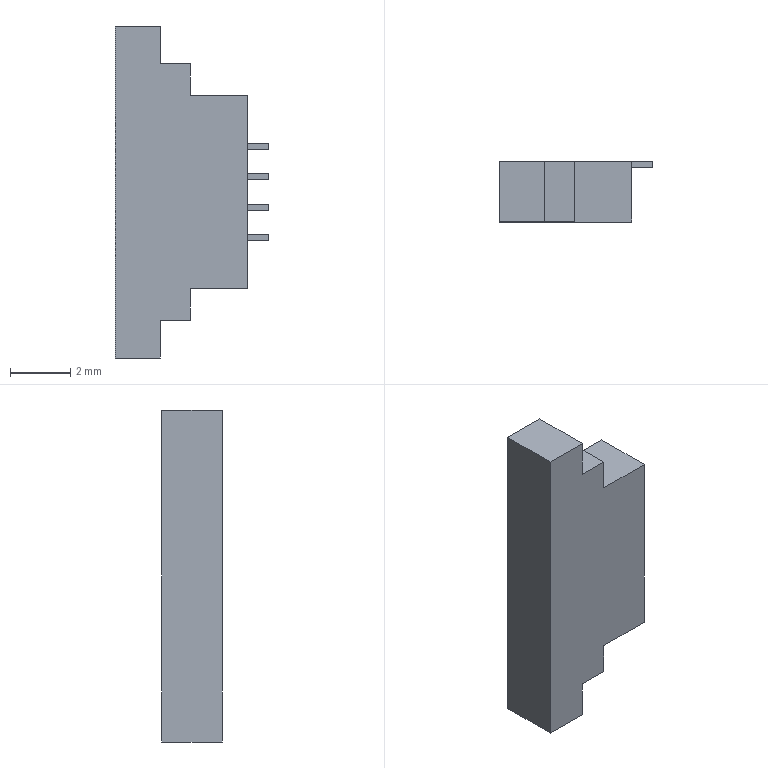Part | SolidWorks | features BaseBody 1 | 1 solid | 30 faces | box 5.1 x 2 x 11 mm | volume 74.432 mm3 | plane 30
STEP:
#1=CARTESIAN_POINT('',(-66.9,-34.61,-10.6));
#2=VERTEX_POINT('',#1);
#3=CARTESIAN_POINT('',(-67.6,-34.61,-10.6));
#4=VERTEX_POINT('',#3);
#5=CARTESIAN_POINT('',(-69.45,-34.61,-10.6));
#6=DIRECTION('',(-1.,0.,0.));
#7=VECTOR('',#6,1000.);
#8=LINE('',#5,#7);
#9=EDGE_CURVE('',#2,#4,#8,.T.);
#10=ORIENTED_EDGE('',*,*,#9,.T.);
#11=CARTESIAN_POINT('',(-67.6,-34.61,-11.4));
#12=VERTEX_POINT('',#11);
#13=CARTESIAN_POINT('',(-67.6,-34.61,-12.));
#14=DIRECTION('',(0.,0.,1.));
#15=VECTOR('',#14,1000.);
#16=LINE('',#13,#15);
#17=EDGE_CURVE('',#12,#4,#16,.T.);
#18=ORIENTED_EDGE('',*,*,#17,.F.);
#19=CARTESIAN_POINT('',(-66.9,-34.61,-11.4));
#20=VERTEX_POINT('',#19);
#21=CARTESIAN_POINT('',(-69.45,-34.61,-11.4));
#22=DIRECTION('',(1.,0.,0.));
#23=VECTOR('',#22,1000.);
#24=LINE('',#21,#23);
#25=EDGE_CURVE('',#12,#20,#24,.T.);
#26=ORIENTED_EDGE('',*,*,#25,.T.);
#27=CARTESIAN_POINT('',(-66.9,-34.61,-11.6));
#28=VERTEX_POINT('',#27);
#29=CARTESIAN_POINT('',(-66.9,-34.61,-12.));
#30=DIRECTION('',(0.,0.,-1.));
#31=VECTOR('',#30,1000.);
#32=LINE('',#29,#31);
#33=EDGE_CURVE('',#20,#28,#32,.T.);
#34=ORIENTED_EDGE('',*,*,#33,.T.);
#35=CARTESIAN_POINT('',(-67.6,-34.61,-11.6));
#36=VERTEX_POINT('',#35);
#37=CARTESIAN_POINT('',(-69.45,-34.61,-11.6));
#38=DIRECTION('',(-1.,0.,0.));
#39=VECTOR('',#38,1000.);
#40=LINE('',#37,#39);
#41=EDGE_CURVE('',#28,#36,#40,.T.);
#42=ORIENTED_EDGE('',*,*,#41,.T.);
#43=CARTESIAN_POINT('',(-67.6,-34.61,-12.4));
#44=VERTEX_POINT('',#43);
#45=CARTESIAN_POINT('',(-67.6,-34.61,-12.));
#46=DIRECTION('',(0.,0.,1.));
#47=VECTOR('',#46,1000.);
#48=LINE('',#45,#47);
#49=EDGE_CURVE('',#44,#36,#48,.T.);
#50=ORIENTED_EDGE('',*,*,#49,.F.);
#51=CARTESIAN_POINT('',(-66.9,-34.61,-12.4));
#52=VERTEX_POINT('',#51);
#53=CARTESIAN_POINT('',(-69.45,-34.61,-12.4));
#54=DIRECTION('',(1.,0.,0.));
#55=VECTOR('',#54,1000.);
#56=LINE('',#53,#55);
#57=EDGE_CURVE('',#44,#52,#56,.T.);
#58=ORIENTED_EDGE('',*,*,#57,.T.);
#59=CARTESIAN_POINT('',(-66.9,-34.61,-12.6));
#60=VERTEX_POINT('',#59);
#61=CARTESIAN_POINT('',(-66.9,-34.61,-12.));
#62=DIRECTION('',(0.,0.,-1.));
#63=VECTOR('',#62,1000.);
#64=LINE('',#61,#63);
#65=EDGE_CURVE('',#52,#60,#64,.T.);
#66=ORIENTED_EDGE('',*,*,#65,.T.);
#67=CARTESIAN_POINT('',(-67.6,-34.61,-12.6));
#68=VERTEX_POINT('',#67);
#69=CARTESIAN_POINT('',(-69.45,-34.61,-12.6));
#70=DIRECTION('',(-1.,0.,0.));
#71=VECTOR('',#70,1000.);
#72=LINE('',#69,#71);
#73=EDGE_CURVE('',#60,#68,#72,.T.);
#74=ORIENTED_EDGE('',*,*,#73,.T.);
#75=CARTESIAN_POINT('',(-67.6,-34.61,-13.4));
#76=VERTEX_POINT('',#75);
#77=CARTESIAN_POINT('',(-67.6,-34.61,-12.));
#78=DIRECTION('',(0.,0.,1.));
#79=VECTOR('',#78,1000.);
#80=LINE('',#77,#79);
#81=EDGE_CURVE('',#76,#68,#80,.T.);
#82=ORIENTED_EDGE('',*,*,#81,.F.);
#83=CARTESIAN_POINT('',(-66.9,-34.61,-13.4));
#84=VERTEX_POINT('',#83);
#85=CARTESIAN_POINT('',(-69.45,-34.61,-13.4));
#86=DIRECTION('',(1.,0.,0.));
#87=VECTOR('',#86,1000.);
#88=LINE('',#85,#87);
#89=EDGE_CURVE('',#76,#84,#88,.T.);
#90=ORIENTED_EDGE('',*,*,#89,.T.);
#91=CARTESIAN_POINT('',(-66.9,-34.61,-13.6));
#92=VERTEX_POINT('',#91);
#93=CARTESIAN_POINT('',(-66.9,-34.61,-12.));
#94=DIRECTION('',(0.,0.,-1.));
#95=VECTOR('',#94,1000.);
#96=LINE('',#93,#95);
#97=EDGE_CURVE('',#84,#92,#96,.T.);
#98=ORIENTED_EDGE('',*,*,#97,.T.);
#99=CARTESIAN_POINT('',(-67.6,-34.61,-13.6));
#100=VERTEX_POINT('',#99);
#101=CARTESIAN_POINT('',(-69.45,-34.61,-13.6));
#102=DIRECTION('',(-1.,0.,0.));
#103=VECTOR('',#102,1000.);
#104=LINE('',#101,#103);
#105=EDGE_CURVE('',#92,#100,#104,.T.);
#106=ORIENTED_EDGE('',*,*,#105,.T.);
#107=CARTESIAN_POINT('',(-67.6,-34.61,-15.2));
#108=VERTEX_POINT('',#107);
#109=CARTESIAN_POINT('',(-67.6,-34.61,-12.));
#110=DIRECTION('',(0.,0.,1.));
#111=VECTOR('',#110,1000.);
#112=LINE('',#109,#111);
#113=EDGE_CURVE('',#108,#100,#112,.T.);
#114=ORIENTED_EDGE('',*,*,#113,.F.);
#115=CARTESIAN_POINT('',(-69.5,-34.61,-15.2));
#116=VERTEX_POINT('',#115);
#117=CARTESIAN_POINT('',(-69.45,-34.61,-15.2));
#118=DIRECTION('',(-1.,0.,0.));
#119=VECTOR('',#118,1000.);
#120=LINE('',#117,#119);
#121=EDGE_CURVE('',#108,#116,#120,.T.);
#122=ORIENTED_EDGE('',*,*,#121,.T.);
#123=CARTESIAN_POINT('',(-69.5,-34.61,-16.25));
#124=VERTEX_POINT('',#123);
#125=CARTESIAN_POINT('',(-69.5,-34.61,-15.725));
#126=DIRECTION('',(0.,0.,1.));
#127=VECTOR('',#126,1000.);
#128=LINE('',#125,#127);
#129=EDGE_CURVE('',#124,#116,#128,.T.);
#130=ORIENTED_EDGE('',*,*,#129,.F.);
#131=CARTESIAN_POINT('',(-70.5,-34.61,-16.25));
#132=VERTEX_POINT('',#131);
#133=CARTESIAN_POINT('',(-70.,-34.61,-16.25));
#134=DIRECTION('',(-1.,0.,0.));
#135=VECTOR('',#134,1000.);
#136=LINE('',#133,#135);
#137=EDGE_CURVE('',#124,#132,#136,.T.);
#138=ORIENTED_EDGE('',*,*,#137,.T.);
#139=CARTESIAN_POINT('',(-70.5,-34.61,-17.5));
#140=VERTEX_POINT('',#139);
#141=CARTESIAN_POINT('',(-70.5,-34.61,-16.875));
#142=DIRECTION('',(0.,0.,1.));
#143=VECTOR('',#142,1000.);
#144=LINE('',#141,#143);
#145=EDGE_CURVE('',#140,#132,#144,.T.);
#146=ORIENTED_EDGE('',*,*,#145,.F.);
#147=CARTESIAN_POINT('',(-72.,-34.61,-17.5));
#148=VERTEX_POINT('',#147);
#149=CARTESIAN_POINT('',(-71.25,-34.61,-17.5));
#150=DIRECTION('',(-1.,0.,0.));
#151=VECTOR('',#150,1000.);
#152=LINE('',#149,#151);
#153=EDGE_CURVE('',#140,#148,#152,.T.);
#154=ORIENTED_EDGE('',*,*,#153,.T.);
#155=CARTESIAN_POINT('',(-72.,-34.61,-6.5));
#156=VERTEX_POINT('',#155);
#157=CARTESIAN_POINT('',(-72.,-34.61,-12.));
#158=DIRECTION('',(0.,0.,1.));
#159=VECTOR('',#158,1000.);
#160=LINE('',#157,#159);
#161=EDGE_CURVE('',#148,#156,#160,.T.);
#162=ORIENTED_EDGE('',*,*,#161,.T.);
#163=CARTESIAN_POINT('',(-70.5,-34.61,-6.5));
#164=VERTEX_POINT('',#163);
#165=CARTESIAN_POINT('',(-71.25,-34.61,-6.5));
#166=DIRECTION('',(-1.,0.,0.));
#167=VECTOR('',#166,1000.);
#168=LINE('',#165,#167);
#169=EDGE_CURVE('',#164,#156,#168,.T.);
#170=ORIENTED_EDGE('',*,*,#169,.F.);
#171=CARTESIAN_POINT('',(-70.5,-34.61,-7.75));
#172=VERTEX_POINT('',#171);
#173=CARTESIAN_POINT('',(-70.5,-34.61,-7.125));
#174=DIRECTION('',(0.,0.,1.));
#175=VECTOR('',#174,1000.);
#176=LINE('',#173,#175);
#177=EDGE_CURVE('',#172,#164,#176,.T.);
#178=ORIENTED_EDGE('',*,*,#177,.F.);
#179=CARTESIAN_POINT('',(-69.5,-34.61,-7.75));
#180=VERTEX_POINT('',#179);
#181=CARTESIAN_POINT('',(-70.,-34.61,-7.75));
#182=DIRECTION('',(-1.,0.,0.));
#183=VECTOR('',#182,1000.);
#184=LINE('',#181,#183);
#185=EDGE_CURVE('',#180,#172,#184,.T.);
#186=ORIENTED_EDGE('',*,*,#185,.F.);
#187=CARTESIAN_POINT('',(-69.5,-34.61,-8.8));
#188=VERTEX_POINT('',#187);
#189=CARTESIAN_POINT('',(-69.5,-34.61,-8.275));
#190=DIRECTION('',(0.,0.,1.));
#191=VECTOR('',#190,1000.);
#192=LINE('',#189,#191);
#193=EDGE_CURVE('',#188,#180,#192,.T.);
#194=ORIENTED_EDGE('',*,*,#193,.F.);
#195=CARTESIAN_POINT('',(-67.6,-34.61,-8.8));
#196=VERTEX_POINT('',#195);
#197=CARTESIAN_POINT('',(-69.45,-34.61,-8.8));
#198=DIRECTION('',(1.,0.,0.));
#199=VECTOR('',#198,1000.);
#200=LINE('',#197,#199);
#201=EDGE_CURVE('',#188,#196,#200,.T.);
#202=ORIENTED_EDGE('',*,*,#201,.T.);
#203=CARTESIAN_POINT('',(-67.6,-34.61,-10.4));
#204=VERTEX_POINT('',#203);
#205=CARTESIAN_POINT('',(-67.6,-34.61,-12.));
#206=DIRECTION('',(0.,0.,1.));
#207=VECTOR('',#206,1000.);
#208=LINE('',#205,#207);
#209=EDGE_CURVE('',#204,#196,#208,.T.);
#210=ORIENTED_EDGE('',*,*,#209,.F.);
#211=CARTESIAN_POINT('',(-66.9,-34.61,-10.4));
#212=VERTEX_POINT('',#211);
#213=CARTESIAN_POINT('',(-69.45,-34.61,-10.4));
#214=DIRECTION('',(1.,0.,0.));
#215=VECTOR('',#214,1000.);
#216=LINE('',#213,#215);
#217=EDGE_CURVE('',#204,#212,#216,.T.);
#218=ORIENTED_EDGE('',*,*,#217,.T.);
#219=CARTESIAN_POINT('',(-66.9,-34.61,-12.));
#220=DIRECTION('',(0.,0.,-1.));
#221=VECTOR('',#220,1000.);
#222=LINE('',#219,#221);
#223=EDGE_CURVE('',#212,#2,#222,.T.);
#224=ORIENTED_EDGE('',*,*,#223,.T.);
#225=EDGE_LOOP('',(#10,#18,#26,#34,#42,#50,#58,#66,#74,#82,#90,#98,#106,#114,#122,#130,#138,#146,#154,#162,#170,#178,#186,#194,#202,#210,#218,#224));
#226=FACE_OUTER_BOUND('',#225,.T.);
#227=CARTESIAN_POINT('',(-69.45,-34.61,-12.));
#228=DIRECTION('',(0.,1.,0.));
#229=DIRECTION('',(0.,0.,1.));
#230=AXIS2_PLACEMENT_3D('',#227,#228,#229);
#231=PLANE('',#230);
#232=ADVANCED_FACE('',(#226),#231,.T.);
#233=CARTESIAN_POINT('',(-66.9,-34.81,-10.6));
#234=VERTEX_POINT('',#233);
#235=CARTESIAN_POINT('',(-66.9,-34.71,-10.6));
#236=DIRECTION('',(0.,1.,0.));
#237=VECTOR('',#236,1000.);
#238=LINE('',#235,#237);
#239=EDGE_CURVE('',#234,#2,#238,.T.);
#240=ORIENTED_EDGE('',*,*,#239,.F.);
#241=CARTESIAN_POINT('',(-67.6,-34.81,-10.6));
#242=VERTEX_POINT('',#241);
#243=CARTESIAN_POINT('',(-67.25,-34.81,-10.6));
#244=DIRECTION('',(1.,0.,0.));
#245=VECTOR('',#244,1000.);
#246=LINE('',#243,#245);
#247=EDGE_CURVE('',#242,#234,#246,.T.);
#248=ORIENTED_EDGE('',*,*,#247,.F.);
#249=CARTESIAN_POINT('',(-67.6,-35.61,-10.6));
#250=DIRECTION('',(0.,-1.,0.));
#251=VECTOR('',#250,1000.);
#252=LINE('',#249,#251);
#253=EDGE_CURVE('',#4,#242,#252,.T.);
#254=ORIENTED_EDGE('',*,*,#253,.F.);
#255=ORIENTED_EDGE('',*,*,#9,.F.);
#256=EDGE_LOOP('',(#240,#248,#254,#255));
#257=FACE_OUTER_BOUND('',#256,.T.);
#258=CARTESIAN_POINT('',(-67.25,-34.71,-10.6));
#259=DIRECTION('',(0.,0.,1.));
#260=DIRECTION('',(1.,0.,0.));
#261=AXIS2_PLACEMENT_3D('',#258,#259,#260);
#262=PLANE('',#261);
#263=ADVANCED_FACE('',(#257),#262,.F.);
#264=ORIENTED_EDGE('',*,*,#239,.T.);
#265=ORIENTED_EDGE('',*,*,#223,.F.);
#266=CARTESIAN_POINT('',(-66.9,-34.81,-10.4));
#267=VERTEX_POINT('',#266);
#268=CARTESIAN_POINT('',(-66.9,-34.71,-10.4));
#269=DIRECTION('',(0.,-1.,0.));
#270=VECTOR('',#269,1000.);
#271=LINE('',#268,#270);
#272=EDGE_CURVE('',#212,#267,#271,.T.);
#273=ORIENTED_EDGE('',*,*,#272,.T.);
#274=CARTESIAN_POINT('',(-66.9,-34.81,-10.5));
#275=DIRECTION('',(0.,0.,-1.));
#276=VECTOR('',#275,1000.);
#277=LINE('',#274,#276);
#278=EDGE_CURVE('',#267,#234,#277,.T.);
#279=ORIENTED_EDGE('',*,*,#278,.T.);
#280=EDGE_LOOP('',(#264,#265,#273,#279));
#281=FACE_OUTER_BOUND('',#280,.T.);
#282=CARTESIAN_POINT('',(-66.9,-34.71,-10.5));
#283=DIRECTION('',(1.,0.,0.));
#284=DIRECTION('',(0.,0.,-1.));
#285=AXIS2_PLACEMENT_3D('',#282,#283,#284);
#286=PLANE('',#285);
#287=ADVANCED_FACE('',(#281),#286,.T.);
#288=ORIENTED_EDGE('',*,*,#217,.F.);
#289=CARTESIAN_POINT('',(-67.6,-34.81,-10.4));
#290=VERTEX_POINT('',#289);
#291=CARTESIAN_POINT('',(-67.6,-35.61,-10.4));
#292=DIRECTION('',(0.,1.,0.));
#293=VECTOR('',#292,1000.);
#294=LINE('',#291,#293);
#295=EDGE_CURVE('',#290,#204,#294,.T.);
#296=ORIENTED_EDGE('',*,*,#295,.F.);
#297=CARTESIAN_POINT('',(-67.25,-34.81,-10.4));
#298=DIRECTION('',(1.,0.,0.));
#299=VECTOR('',#298,1000.);
#300=LINE('',#297,#299);
#301=EDGE_CURVE('',#290,#267,#300,.T.);
#302=ORIENTED_EDGE('',*,*,#301,.T.);
#303=ORIENTED_EDGE('',*,*,#272,.F.);
#304=EDGE_LOOP('',(#288,#296,#302,#303));
#305=FACE_OUTER_BOUND('',#304,.T.);
#306=CARTESIAN_POINT('',(-67.25,-34.71,-10.4));
#307=DIRECTION('',(0.,0.,1.));
#308=DIRECTION('',(1.,0.,0.));
#309=AXIS2_PLACEMENT_3D('',#306,#307,#308);
#310=PLANE('',#309);
#311=ADVANCED_FACE('',(#305),#310,.T.);
#312=CARTESIAN_POINT('',(-69.5,-36.61,-8.8));
#313=VERTEX_POINT('',#312);
#314=CARTESIAN_POINT('',(-67.6,-36.61,-8.8));
#315=VERTEX_POINT('',#314);
#316=CARTESIAN_POINT('',(-68.55,-36.61,-8.8));
#317=DIRECTION('',(1.,0.,0.));
#318=VECTOR('',#317,1000.);
#319=LINE('',#316,#318);
#320=EDGE_CURVE('',#313,#315,#319,.T.);
#321=ORIENTED_EDGE('',*,*,#320,.T.);
#322=CARTESIAN_POINT('',(-67.6,-35.61,-8.8));
#323=DIRECTION('',(0.,1.,0.));
#324=VECTOR('',#323,1000.);
#325=LINE('',#322,#324);
#326=EDGE_CURVE('',#315,#196,#325,.T.);
#327=ORIENTED_EDGE('',*,*,#326,.T.);
#328=ORIENTED_EDGE('',*,*,#201,.F.);
#329=CARTESIAN_POINT('',(-69.5,-35.61,-8.8));
#330=DIRECTION('',(0.,-1.,0.));
#331=VECTOR('',#330,1000.);
#332=LINE('',#329,#331);
#333=EDGE_CURVE('',#188,#313,#332,.T.);
#334=ORIENTED_EDGE('',*,*,#333,.T.);
#335=EDGE_LOOP('',(#321,#327,#328,#334));
#336=FACE_OUTER_BOUND('',#335,.T.);
#337=CARTESIAN_POINT('',(-68.55,-35.61,-8.8));
#338=DIRECTION('',(0.,0.,1.));
#339=DIRECTION('',(1.,0.,0.));
#340=AXIS2_PLACEMENT_3D('',#337,#338,#339);
#341=PLANE('',#340);
#342=ADVANCED_FACE('',(#336),#341,.T.);
#343=CARTESIAN_POINT('',(-72.,-36.61,-6.5));
#344=VERTEX_POINT('',#343);
#345=CARTESIAN_POINT('',(-72.,-35.61,-6.5));
#346=DIRECTION('',(0.,-1.,0.));
#347=VECTOR('',#346,1000.);
#348=LINE('',#345,#347);
#349=EDGE_CURVE('',#156,#344,#348,.T.);
#350=ORIENTED_EDGE('',*,*,#349,.F.);
#351=ORIENTED_EDGE('',*,*,#161,.F.);
#352=CARTESIAN_POINT('',(-72.,-36.61,-17.5));
#353=VERTEX_POINT('',#352);
#354=CARTESIAN_POINT('',(-72.,-35.61,-17.5));
#355=DIRECTION('',(0.,1.,0.));
#356=VECTOR('',#355,1000.);
#357=LINE('',#354,#356);
#358=EDGE_CURVE('',#353,#148,#357,.T.);
#359=ORIENTED_EDGE('',*,*,#358,.F.);
#360=CARTESIAN_POINT('',(-72.,-36.61,-12.));
#361=DIRECTION('',(0.,0.,-1.));
#362=VECTOR('',#361,1000.);
#363=LINE('',#360,#362);
#364=EDGE_CURVE('',#344,#353,#363,.T.);
#365=ORIENTED_EDGE('',*,*,#364,.F.);
#366=EDGE_LOOP('',(#350,#351,#359,#365));
#367=FACE_OUTER_BOUND('',#366,.T.);
#368=CARTESIAN_POINT('',(-72.,-35.61,-12.));
#369=DIRECTION('',(1.,0.,0.));
#370=DIRECTION('',(0.,0.,-1.));
#371=AXIS2_PLACEMENT_3D('',#368,#369,#370);
#372=PLANE('',#371);
#373=ADVANCED_FACE('',(#367),#372,.F.);
#374=CARTESIAN_POINT('',(-69.5,-36.61,-15.2));
#375=VERTEX_POINT('',#374);
#376=CARTESIAN_POINT('',(-69.5,-35.61,-15.2));
#377=DIRECTION('',(0.,-1.,0.));
#378=VECTOR('',#377,1000.);
#379=LINE('',#376,#378);
#380=EDGE_CURVE('',#116,#375,#379,.T.);
#381=ORIENTED_EDGE('',*,*,#380,.F.);
#382=ORIENTED_EDGE('',*,*,#121,.F.);
#383=CARTESIAN_POINT('',(-67.6,-36.61,-15.2));
#384=VERTEX_POINT('',#383);
#385=CARTESIAN_POINT('',(-67.6,-35.61,-15.2));
#386=DIRECTION('',(0.,1.,0.));
#387=VECTOR('',#386,1000.);
#388=LINE('',#385,#387);
#389=EDGE_CURVE('',#384,#108,#388,.T.);
#390=ORIENTED_EDGE('',*,*,#389,.F.);
#391=CARTESIAN_POINT('',(-68.55,-36.61,-15.2));
#392=DIRECTION('',(1.,0.,0.));
#393=VECTOR('',#392,1000.);
#394=LINE('',#391,#393);
#395=EDGE_CURVE('',#375,#384,#394,.T.);
#396=ORIENTED_EDGE('',*,*,#395,.F.);
#397=EDGE_LOOP('',(#381,#382,#390,#396));
#398=FACE_OUTER_BOUND('',#397,.T.);
#399=CARTESIAN_POINT('',(-68.55,-35.61,-15.2));
#400=DIRECTION('',(0.,0.,1.));
#401=DIRECTION('',(1.,0.,0.));
#402=AXIS2_PLACEMENT_3D('',#399,#400,#401);
#403=PLANE('',#402);
#404=ADVANCED_FACE('',(#398),#403,.F.);
#405=CARTESIAN_POINT('',(-66.9,-34.81,-13.6));
#406=VERTEX_POINT('',#405);
#407=CARTESIAN_POINT('',(-66.9,-34.71,-13.6));
#408=DIRECTION('',(0.,1.,0.));
#409=VECTOR('',#408,1000.);
#410=LINE('',#407,#409);
#411=EDGE_CURVE('',#406,#92,#410,.T.);
#412=ORIENTED_EDGE('',*,*,#411,.F.);
#413=CARTESIAN_POINT('',(-67.6,-34.81,-13.6));
#414=VERTEX_POINT('',#413);
#415=CARTESIAN_POINT('',(-67.25,-34.81,-13.6));
#416=DIRECTION('',(1.,0.,0.));
#417=VECTOR('',#416,1000.);
#418=LINE('',#415,#417);
#419=EDGE_CURVE('',#414,#406,#418,.T.);
#420=ORIENTED_EDGE('',*,*,#419,.F.);
#421=CARTESIAN_POINT('',(-67.6,-34.71,-13.6));
#422=DIRECTION('',(0.,-1.,0.));
#423=VECTOR('',#422,1000.);
#424=LINE('',#421,#423);
#425=EDGE_CURVE('',#100,#414,#424,.T.);
#426=ORIENTED_EDGE('',*,*,#425,.F.);
#427=ORIENTED_EDGE('',*,*,#105,.F.);
#428=EDGE_LOOP('',(#412,#420,#426,#427));
#429=FACE_OUTER_BOUND('',#428,.T.);
#430=CARTESIAN_POINT('',(-67.25,-34.71,-13.6));
#431=DIRECTION('',(0.,0.,1.));
#432=DIRECTION('',(1.,0.,0.));
#433=AXIS2_PLACEMENT_3D('',#430,#431,#432);
#434=PLANE('',#433);
#435=ADVANCED_FACE('',(#429),#434,.F.);
#436=ORIENTED_EDGE('',*,*,#411,.T.);
#437=ORIENTED_EDGE('',*,*,#97,.F.);
#438=CARTESIAN_POINT('',(-66.9,-34.81,-13.4));
#439=VERTEX_POINT('',#438);
#440=CARTESIAN_POINT('',(-66.9,-34.71,-13.4));
#441=DIRECTION('',(0.,-1.,0.));
#442=VECTOR('',#441,1000.);
#443=LINE('',#440,#442);
#444=EDGE_CURVE('',#84,#439,#443,.T.);
#445=ORIENTED_EDGE('',*,*,#444,.T.);
#446=CARTESIAN_POINT('',(-66.9,-34.81,-13.5));
#447=DIRECTION('',(0.,0.,-1.));
#448=VECTOR('',#447,1000.);
#449=LINE('',#446,#448);
#450=EDGE_CURVE('',#439,#406,#449,.T.);
#451=ORIENTED_EDGE('',*,*,#450,.T.);
#452=EDGE_LOOP('',(#436,#437,#445,#451));
#453=FACE_OUTER_BOUND('',#452,.T.);
#454=CARTESIAN_POINT('',(-66.9,-34.71,-13.5));
#455=DIRECTION('',(1.,0.,0.));
#456=DIRECTION('',(0.,0.,-1.));
#457=AXIS2_PLACEMENT_3D('',#454,#455,#456);
#458=PLANE('',#457);
#459=ADVANCED_FACE('',(#453),#458,.T.);
#460=ORIENTED_EDGE('',*,*,#89,.F.);
#461=CARTESIAN_POINT('',(-67.6,-34.81,-13.4));
#462=VERTEX_POINT('',#461);
#463=CARTESIAN_POINT('',(-67.6,-34.71,-13.4));
#464=DIRECTION('',(0.,-1.,0.));
#465=VECTOR('',#464,1000.);
#466=LINE('',#463,#465);
#467=EDGE_CURVE('',#76,#462,#466,.T.);
#468=ORIENTED_EDGE('',*,*,#467,.T.);
#469=CARTESIAN_POINT('',(-67.25,-34.81,-13.4));
#470=DIRECTION('',(1.,0.,0.));
#471=VECTOR('',#470,1000.);
#472=LINE('',#469,#471);
#473=EDGE_CURVE('',#462,#439,#472,.T.);
#474=ORIENTED_EDGE('',*,*,#473,.T.);
#475=ORIENTED_EDGE('',*,*,#444,.F.);
#476=EDGE_LOOP('',(#460,#468,#474,#475));
#477=FACE_OUTER_BOUND('',#476,.T.);
#478=CARTESIAN_POINT('',(-67.25,-34.71,-13.4));
#479=DIRECTION('',(0.,0.,1.));
#480=DIRECTION('',(1.,0.,0.));
#481=AXIS2_PLACEMENT_3D('',#478,#479,#480);
#482=PLANE('',#481);
#483=ADVANCED_FACE('',(#477),#482,.T.);
#484=CARTESIAN_POINT('',(-66.9,-34.81,-12.6));
#485=VERTEX_POINT('',#484);
#486=CARTESIAN_POINT('',(-66.9,-34.71,-12.6));
#487=DIRECTION('',(0.,1.,0.));
#488=VECTOR('',#487,1000.);
#489=LINE('',#486,#488);
#490=EDGE_CURVE('',#485,#60,#489,.T.);
#491=ORIENTED_EDGE('',*,*,#490,.F.);
#492=CARTESIAN_POINT('',(-67.6,-34.81,-12.6));
#493=VERTEX_POINT('',#492);
#494=CARTESIAN_POINT('',(-67.25,-34.81,-12.6));
#495=DIRECTION('',(1.,0.,0.));
#496=VECTOR('',#495,1000.);
#497=LINE('',#494,#496);
#498=EDGE_CURVE('',#493,#485,#497,.T.);
#499=ORIENTED_EDGE('',*,*,#498,.F.);
#500=CARTESIAN_POINT('',(-67.6,-34.71,-12.6));
#501=DIRECTION('',(0.,-1.,0.));
#502=VECTOR('',#501,1000.);
#503=LINE('',#500,#502);
#504=EDGE_CURVE('',#68,#493,#503,.T.);
#505=ORIENTED_EDGE('',*,*,#504,.F.);
#506=ORIENTED_EDGE('',*,*,#73,.F.);
#507=EDGE_LOOP('',(#491,#499,#505,#506));
#508=FACE_OUTER_BOUND('',#507,.T.);
#509=CARTESIAN_POINT('',(-67.25,-34.71,-12.6));
#510=DIRECTION('',(0.,0.,1.));
#511=DIRECTION('',(1.,0.,0.));
#512=AXIS2_PLACEMENT_3D('',#509,#510,#511);
#513=PLANE('',#512);
#514=ADVANCED_FACE('',(#508),#513,.F.);
#515=ORIENTED_EDGE('',*,*,#490,.T.);
#516=ORIENTED_EDGE('',*,*,#65,.F.);
#517=CARTESIAN_POINT('',(-66.9,-34.81,-12.4));
#518=VERTEX_POINT('',#517);
#519=CARTESIAN_POINT('',(-66.9,-34.71,-12.4));
#520=DIRECTION('',(0.,-1.,0.));
#521=VECTOR('',#520,1000.);
#522=LINE('',#519,#521);
#523=EDGE_CURVE('',#52,#518,#522,.T.);
#524=ORIENTED_EDGE('',*,*,#523,.T.);
#525=CARTESIAN_POINT('',(-66.9,-34.81,-12.5));
#526=DIRECTION('',(0.,0.,-1.));
#527=VECTOR('',#526,1000.);
#528=LINE('',#525,#527);
#529=EDGE_CURVE('',#518,#485,#528,.T.);
#530=ORIENTED_EDGE('',*,*,#529,.T.);
#531=EDGE_LOOP('',(#515,#516,#524,#530));
#532=FACE_OUTER_BOUND('',#531,.T.);
#533=CARTESIAN_POINT('',(-66.9,-34.71,-12.5));
#534=DIRECTION('',(1.,0.,0.));
#535=DIRECTION('',(0.,0.,-1.));
#536=AXIS2_PLACEMENT_3D('',#533,#534,#535);
#537=PLANE('',#536);
#538=ADVANCED_FACE('',(#532),#537,.T.);
#539=ORIENTED_EDGE('',*,*,#57,.F.);
#540=CARTESIAN_POINT('',(-67.6,-34.81,-12.4));
#541=VERTEX_POINT('',#540);
#542=CARTESIAN_POINT('',(-67.6,-34.71,-12.4));
#543=DIRECTION('',(0.,-1.,0.));
#544=VECTOR('',#543,1000.);
#545=LINE('',#542,#544);
#546=EDGE_CURVE('',#44,#541,#545,.T.);
#547=ORIENTED_EDGE('',*,*,#546,.T.);
#548=CARTESIAN_POINT('',(-67.25,-34.81,-12.4));
#549=DIRECTION('',(1.,0.,0.));
#550=VECTOR('',#549,1000.);
#551=LINE('',#548,#550);
#552=EDGE_CURVE('',#541,#518,#551,.T.);
#553=ORIENTED_EDGE('',*,*,#552,.T.);
#554=ORIENTED_EDGE('',*,*,#523,.F.);
#555=EDGE_LOOP('',(#539,#547,#553,#554));
#556=FACE_OUTER_BOUND('',#555,.T.);
#557=CARTESIAN_POINT('',(-67.25,-34.71,-12.4));
#558=DIRECTION('',(0.,0.,1.));
#559=DIRECTION('',(1.,0.,0.));
#560=AXIS2_PLACEMENT_3D('',#557,#558,#559);
#561=PLANE('',#560);
#562=ADVANCED_FACE('',(#556),#561,.T.);
#563=CARTESIAN_POINT('',(-66.9,-34.81,-11.6));
#564=VERTEX_POINT('',#563);
#565=CARTESIAN_POINT('',(-66.9,-34.71,-11.6));
#566=DIRECTION('',(0.,1.,0.));
#567=VECTOR('',#566,1000.);
#568=LINE('',#565,#567);
#569=EDGE_CURVE('',#564,#28,#568,.T.);
#570=ORIENTED_EDGE('',*,*,#569,.F.);
#571=CARTESIAN_POINT('',(-67.6,-34.81,-11.6));
#572=VERTEX_POINT('',#571);
#573=CARTESIAN_POINT('',(-67.25,-34.81,-11.6));
#574=DIRECTION('',(1.,0.,0.));
#575=VECTOR('',#574,1000.);
#576=LINE('',#573,#575);
#577=EDGE_CURVE('',#572,#564,#576,.T.);
#578=ORIENTED_EDGE('',*,*,#577,.F.);
#579=CARTESIAN_POINT('',(-67.6,-34.71,-11.6));
#580=DIRECTION('',(0.,-1.,0.));
#581=VECTOR('',#580,1000.);
#582=LINE('',#579,#581);
#583=EDGE_CURVE('',#36,#572,#582,.T.);
#584=ORIENTED_EDGE('',*,*,#583,.F.);
#585=ORIENTED_EDGE('',*,*,#41,.F.);
#586=EDGE_LOOP('',(#570,#578,#584,#585));
#587=FACE_OUTER_BOUND('',#586,.T.);
#588=CARTESIAN_POINT('',(-67.25,-34.71,-11.6));
#589=DIRECTION('',(0.,0.,1.));
#590=DIRECTION('',(1.,0.,0.));
#591=AXIS2_PLACEMENT_3D('',#588,#589,#590);
#592=PLANE('',#591);
#593=ADVANCED_FACE('',(#587),#592,.F.);
#594=ORIENTED_EDGE('',*,*,#569,.T.);
#595=ORIENTED_EDGE('',*,*,#33,.F.);
#596=CARTESIAN_POINT('',(-66.9,-34.81,-11.4));
#597=VERTEX_POINT('',#596);
#598=CARTESIAN_POINT('',(-66.9,-34.71,-11.4));
#599=DIRECTION('',(0.,-1.,0.));
#600=VECTOR('',#599,1000.);
#601=LINE('',#598,#600);
#602=EDGE_CURVE('',#20,#597,#601,.T.);
#603=ORIENTED_EDGE('',*,*,#602,.T.);
#604=CARTESIAN_POINT('',(-66.9,-34.81,-11.5));
#605=DIRECTION('',(0.,0.,-1.));
#606=VECTOR('',#605,1000.);
#607=LINE('',#604,#606);
#608=EDGE_CURVE('',#597,#564,#607,.T.);
#609=ORIENTED_EDGE('',*,*,#608,.T.);
#610=EDGE_LOOP('',(#594,#595,#603,#609));
#611=FACE_OUTER_BOUND('',#610,.T.);
#612=CARTESIAN_POINT('',(-66.9,-34.71,-11.5));
#613=DIRECTION('',(1.,0.,0.));
#614=DIRECTION('',(0.,0.,-1.));
#615=AXIS2_PLACEMENT_3D('',#612,#613,#614);
#616=PLANE('',#615);
#617=ADVANCED_FACE('',(#611),#616,.T.);
#618=ORIENTED_EDGE('',*,*,#25,.F.);
#619=CARTESIAN_POINT('',(-67.6,-34.81,-11.4));
#620=VERTEX_POINT('',#619);
#621=CARTESIAN_POINT('',(-67.6,-34.71,-11.4));
#622=DIRECTION('',(0.,-1.,0.));
#623=VECTOR('',#622,1000.);
#624=LINE('',#621,#623);
#625=EDGE_CURVE('',#12,#620,#624,.T.);
#626=ORIENTED_EDGE('',*,*,#625,.T.);
#627=CARTESIAN_POINT('',(-67.25,-34.81,-11.4));
#628=DIRECTION('',(1.,0.,0.));
#629=VECTOR('',#628,1000.);
#630=LINE('',#627,#629);
#631=EDGE_CURVE('',#620,#597,#630,.T.);
#632=ORIENTED_EDGE('',*,*,#631,.T.);
#633=ORIENTED_EDGE('',*,*,#602,.F.);
#634=EDGE_LOOP('',(#618,#626,#632,#633));
#635=FACE_OUTER_BOUND('',#634,.T.);
#636=CARTESIAN_POINT('',(-67.25,-34.71,-11.4));
#637=DIRECTION('',(0.,0.,1.));
#638=DIRECTION('',(1.,0.,0.));
#639=AXIS2_PLACEMENT_3D('',#636,#637,#638);
#640=PLANE('',#639);
#641=ADVANCED_FACE('',(#635),#640,.T.);
#642=ORIENTED_EDGE('',*,*,#278,.F.);
#643=ORIENTED_EDGE('',*,*,#301,.F.);
#644=CARTESIAN_POINT('',(-67.6,-34.81,-10.5));
#645=DIRECTION('',(0.,0.,1.));
#646=VECTOR('',#645,1000.);
#647=LINE('',#644,#646);
#648=EDGE_CURVE('',#242,#290,#647,.T.);
#649=ORIENTED_EDGE('',*,*,#648,.F.);
#650=ORIENTED_EDGE('',*,*,#247,.T.);
#651=EDGE_LOOP('',(#642,#643,#649,#650));
#652=FACE_OUTER_BOUND('',#651,.T.);
#653=CARTESIAN_POINT('',(-67.25,-34.81,-10.5));
#654=DIRECTION('',(0.,1.,0.));
#655=DIRECTION('',(0.,0.,1.));
#656=AXIS2_PLACEMENT_3D('',#653,#654,#655);
#657=PLANE('',#656);
#658=ADVANCED_FACE('',(#652),#657,.F.);
#659=ORIENTED_EDGE('',*,*,#425,.T.);
#660=CARTESIAN_POINT('',(-67.6,-34.81,-12.));
#661=DIRECTION('',(0.,0.,1.));
#662=VECTOR('',#661,1000.);
#663=LINE('',#660,#662);
#664=EDGE_CURVE('',#414,#462,#663,.T.);
#665=ORIENTED_EDGE('',*,*,#664,.T.);
#666=ORIENTED_EDGE('',*,*,#467,.F.);
#667=ORIENTED_EDGE('',*,*,#81,.T.);
#668=ORIENTED_EDGE('',*,*,#504,.T.);
#669=CARTESIAN_POINT('',(-67.6,-34.81,-12.));
#670=DIRECTION('',(0.,0.,1.));
#671=VECTOR('',#670,1000.);
#672=LINE('',#669,#671);
#673=EDGE_CURVE('',#493,#541,#672,.T.);
#674=ORIENTED_EDGE('',*,*,#673,.T.);
#675=ORIENTED_EDGE('',*,*,#546,.F.);
#676=ORIENTED_EDGE('',*,*,#49,.T.);
#677=ORIENTED_EDGE('',*,*,#583,.T.);
#678=CARTESIAN_POINT('',(-67.6,-34.81,-12.));
#679=DIRECTION('',(0.,0.,1.));
#680=VECTOR('',#679,1000.);
#681=LINE('',#678,#680);
#682=EDGE_CURVE('',#572,#620,#681,.T.);
#683=ORIENTED_EDGE('',*,*,#682,.T.);
#684=ORIENTED_EDGE('',*,*,#625,.F.);
#685=ORIENTED_EDGE('',*,*,#17,.T.);
#686=ORIENTED_EDGE('',*,*,#253,.T.);
#687=ORIENTED_EDGE('',*,*,#648,.T.);
#688=ORIENTED_EDGE('',*,*,#295,.T.);
#689=ORIENTED_EDGE('',*,*,#209,.T.);
#690=ORIENTED_EDGE('',*,*,#326,.F.);
#691=CARTESIAN_POINT('',(-67.6,-36.61,-12.));
#692=DIRECTION('',(0.,0.,-1.));
#693=VECTOR('',#692,1000.);
#694=LINE('',#691,#693);
#695=EDGE_CURVE('',#315,#384,#694,.T.);
#696=ORIENTED_EDGE('',*,*,#695,.T.);
#697=ORIENTED_EDGE('',*,*,#389,.T.);
#698=ORIENTED_EDGE('',*,*,#113,.T.);
#699=EDGE_LOOP('',(#659,#665,#666,#667,#668,#674,#675,#676,#677,#683,#684,#685,#686,#687,#688,#689,#690,#696,#697,#698));
#700=FACE_OUTER_BOUND('',#699,.T.);
#701=CARTESIAN_POINT('',(-67.6,-35.61,-12.));
#702=DIRECTION('',(1.,0.,0.));
#703=DIRECTION('',(0.,0.,-1.));
#704=AXIS2_PLACEMENT_3D('',#701,#702,#703);
#705=PLANE('',#704);
#706=ADVANCED_FACE('',(#700),#705,.T.);
#707=CARTESIAN_POINT('',(-70.5,-36.61,-7.75));
#708=VERTEX_POINT('',#707);
#709=CARTESIAN_POINT('',(-69.5,-36.61,-7.75));
#710=VERTEX_POINT('',#709);
#711=CARTESIAN_POINT('',(-70.,-36.61,-7.75));
#712=DIRECTION('',(1.,0.,0.));
#713=VECTOR('',#712,1000.);
#714=LINE('',#711,#713);
#715=EDGE_CURVE('',#708,#710,#714,.T.);
#716=ORIENTED_EDGE('',*,*,#715,.F.);
#717=CARTESIAN_POINT('',(-70.5,-36.61,-6.5));
#718=VERTEX_POINT('',#717);
#719=CARTESIAN_POINT('',(-70.5,-36.61,-7.125));
#720=DIRECTION('',(0.,0.,-1.));
#721=VECTOR('',#720,1000.);
#722=LINE('',#719,#721);
#723=EDGE_CURVE('',#718,#708,#722,.T.);
#724=ORIENTED_EDGE('',*,*,#723,.F.);
#725=CARTESIAN_POINT('',(-69.8,-36.61,-6.5));
#726=DIRECTION('',(1.,0.,0.));
#727=VECTOR('',#726,1000.);
#728=LINE('',#725,#727);
#729=EDGE_CURVE('',#344,#718,#728,.T.);
#730=ORIENTED_EDGE('',*,*,#729,.F.);
#731=ORIENTED_EDGE('',*,*,#364,.T.);
#732=CARTESIAN_POINT('',(-70.5,-36.61,-17.5));
#733=VERTEX_POINT('',#732);
#734=CARTESIAN_POINT('',(-69.8,-36.61,-17.5));
#735=DIRECTION('',(-1.,0.,0.));
#736=VECTOR('',#735,1000.);
#737=LINE('',#734,#736);
#738=EDGE_CURVE('',#733,#353,#737,.T.);
#739=ORIENTED_EDGE('',*,*,#738,.F.);
#740=CARTESIAN_POINT('',(-70.5,-36.61,-16.25));
#741=VERTEX_POINT('',#740);
#742=CARTESIAN_POINT('',(-70.5,-36.61,-16.875));
#743=DIRECTION('',(0.,0.,-1.));
#744=VECTOR('',#743,1000.);
#745=LINE('',#742,#744);
#746=EDGE_CURVE('',#741,#733,#745,.T.);
#747=ORIENTED_EDGE('',*,*,#746,.F.);
#748=CARTESIAN_POINT('',(-69.5,-36.61,-16.25));
#749=VERTEX_POINT('',#748);
#750=CARTESIAN_POINT('',(-70.,-36.61,-16.25));
#751=DIRECTION('',(1.,0.,0.));
#752=VECTOR('',#751,1000.);
#753=LINE('',#750,#752);
#754=EDGE_CURVE('',#741,#749,#753,.T.);
#755=ORIENTED_EDGE('',*,*,#754,.T.);
#756=CARTESIAN_POINT('',(-69.5,-36.61,-12.));
#757=DIRECTION('',(0.,0.,-1.));
#758=VECTOR('',#757,1000.);
#759=LINE('',#756,#758);
#760=EDGE_CURVE('',#375,#749,#759,.T.);
#761=ORIENTED_EDGE('',*,*,#760,.F.);
#762=ORIENTED_EDGE('',*,*,#395,.T.);
#763=ORIENTED_EDGE('',*,*,#695,.F.);
#764=ORIENTED_EDGE('',*,*,#320,.F.);
#765=CARTESIAN_POINT('',(-69.5,-36.61,-12.));
#766=DIRECTION('',(0.,0.,-1.));
#767=VECTOR('',#766,1000.);
#768=LINE('',#765,#767);
#769=EDGE_CURVE('',#710,#313,#768,.T.);
#770=ORIENTED_EDGE('',*,*,#769,.F.);
#771=EDGE_LOOP('',(#716,#724,#730,#731,#739,#747,#755,#761,#762,#763,#764,#770));
#772=FACE_OUTER_BOUND('',#771,.T.);
#773=CARTESIAN_POINT('',(-69.8,-36.61,-12.));
#774=DIRECTION('',(0.,1.,0.));
#775=DIRECTION('',(0.,0.,1.));
#776=AXIS2_PLACEMENT_3D('',#773,#774,#775);
#777=PLANE('',#776);
#778=ADVANCED_FACE('',(#772),#777,.F.);
#779=CARTESIAN_POINT('',(-69.5,-35.61,-7.75));
#780=DIRECTION('',(0.,-1.,0.));
#781=VECTOR('',#780,1000.);
#782=LINE('',#779,#781);
#783=EDGE_CURVE('',#180,#710,#782,.T.);
#784=ORIENTED_EDGE('',*,*,#783,.T.);
#785=ORIENTED_EDGE('',*,*,#769,.T.);
#786=ORIENTED_EDGE('',*,*,#333,.F.);
#787=ORIENTED_EDGE('',*,*,#193,.T.);
#788=EDGE_LOOP('',(#784,#785,#786,#787));
#789=FACE_OUTER_BOUND('',#788,.T.);
#790=CARTESIAN_POINT('',(-69.5,-35.61,-8.275));
#791=DIRECTION('',(1.,0.,0.));
#792=DIRECTION('',(0.,0.,-1.));
#793=AXIS2_PLACEMENT_3D('',#790,#791,#792);
#794=PLANE('',#793);
#795=ADVANCED_FACE('',(#789),#794,.T.);
#796=ORIENTED_EDGE('',*,*,#729,.T.);
#797=CARTESIAN_POINT('',(-70.5,-35.61,-6.5));
#798=DIRECTION('',(0.,1.,0.));
#799=VECTOR('',#798,1000.);
#800=LINE('',#797,#799);
#801=EDGE_CURVE('',#718,#164,#800,.T.);
#802=ORIENTED_EDGE('',*,*,#801,.T.);
#803=ORIENTED_EDGE('',*,*,#169,.T.);
#804=ORIENTED_EDGE('',*,*,#349,.T.);
#805=EDGE_LOOP('',(#796,#802,#803,#804));
#806=FACE_OUTER_BOUND('',#805,.T.);
#807=CARTESIAN_POINT('',(-71.25,-35.61,-6.5));
#808=DIRECTION('',(0.,0.,1.));
#809=DIRECTION('',(1.,0.,0.));
#810=AXIS2_PLACEMENT_3D('',#807,#808,#809);
#811=PLANE('',#810);
#812=ADVANCED_FACE('',(#806),#811,.T.);
#813=ORIENTED_EDGE('',*,*,#358,.T.);
#814=ORIENTED_EDGE('',*,*,#153,.F.);
#815=CARTESIAN_POINT('',(-70.5,-35.61,-17.5));
#816=DIRECTION('',(0.,1.,0.));
#817=VECTOR('',#816,1000.);
#818=LINE('',#815,#817);
#819=EDGE_CURVE('',#733,#140,#818,.T.);
#820=ORIENTED_EDGE('',*,*,#819,.F.);
#821=ORIENTED_EDGE('',*,*,#738,.T.);
#822=EDGE_LOOP('',(#813,#814,#820,#821));
#823=FACE_OUTER_BOUND('',#822,.T.);
#824=CARTESIAN_POINT('',(-71.25,-35.61,-17.5));
#825=DIRECTION('',(0.,0.,1.));
#826=DIRECTION('',(1.,0.,0.));
#827=AXIS2_PLACEMENT_3D('',#824,#825,#826);
#828=PLANE('',#827);
#829=ADVANCED_FACE('',(#823),#828,.F.);
#830=ORIENTED_EDGE('',*,*,#380,.T.);
#831=ORIENTED_EDGE('',*,*,#760,.T.);
#832=CARTESIAN_POINT('',(-69.5,-35.61,-16.25));
#833=DIRECTION('',(0.,1.,0.));
#834=VECTOR('',#833,1000.);
#835=LINE('',#832,#834);
#836=EDGE_CURVE('',#749,#124,#835,.T.);
#837=ORIENTED_EDGE('',*,*,#836,.T.);
#838=ORIENTED_EDGE('',*,*,#129,.T.);
#839=EDGE_LOOP('',(#830,#831,#837,#838));
#840=FACE_OUTER_BOUND('',#839,.T.);
#841=CARTESIAN_POINT('',(-69.5,-35.61,-15.725));
#842=DIRECTION('',(1.,0.,0.));
#843=DIRECTION('',(0.,0.,-1.));
#844=AXIS2_PLACEMENT_3D('',#841,#842,#843);
#845=PLANE('',#844);
#846=ADVANCED_FACE('',(#840),#845,.T.);
#847=ORIENTED_EDGE('',*,*,#450,.F.);
#848=ORIENTED_EDGE('',*,*,#473,.F.);
#849=ORIENTED_EDGE('',*,*,#664,.F.);
#850=ORIENTED_EDGE('',*,*,#419,.T.);
#851=EDGE_LOOP('',(#847,#848,#849,#850));
#852=FACE_OUTER_BOUND('',#851,.T.);
#853=CARTESIAN_POINT('',(-67.25,-34.81,-13.5));
#854=DIRECTION('',(0.,1.,0.));
#855=DIRECTION('',(0.,0.,1.));
#856=AXIS2_PLACEMENT_3D('',#853,#854,#855);
#857=PLANE('',#856);
#858=ADVANCED_FACE('',(#852),#857,.F.);
#859=ORIENTED_EDGE('',*,*,#529,.F.);
#860=ORIENTED_EDGE('',*,*,#552,.F.);
#861=ORIENTED_EDGE('',*,*,#673,.F.);
#862=ORIENTED_EDGE('',*,*,#498,.T.);
#863=EDGE_LOOP('',(#859,#860,#861,#862));
#864=FACE_OUTER_BOUND('',#863,.T.);
#865=CARTESIAN_POINT('',(-67.25,-34.81,-12.5));
#866=DIRECTION('',(0.,1.,0.));
#867=DIRECTION('',(0.,0.,1.));
#868=AXIS2_PLACEMENT_3D('',#865,#866,#867);
#869=PLANE('',#868);
#870=ADVANCED_FACE('',(#864),#869,.F.);
#871=ORIENTED_EDGE('',*,*,#608,.F.);
#872=ORIENTED_EDGE('',*,*,#631,.F.);
#873=ORIENTED_EDGE('',*,*,#682,.F.);
#874=ORIENTED_EDGE('',*,*,#577,.T.);
#875=EDGE_LOOP('',(#871,#872,#873,#874));
#876=FACE_OUTER_BOUND('',#875,.T.);
#877=CARTESIAN_POINT('',(-67.25,-34.81,-11.5));
#878=DIRECTION('',(0.,1.,0.));
#879=DIRECTION('',(0.,0.,1.));
#880=AXIS2_PLACEMENT_3D('',#877,#878,#879);
#881=PLANE('',#880);
#882=ADVANCED_FACE('',(#876),#881,.F.);
#883=ORIENTED_EDGE('',*,*,#715,.T.);
#884=ORIENTED_EDGE('',*,*,#783,.F.);
#885=ORIENTED_EDGE('',*,*,#185,.T.);
#886=CARTESIAN_POINT('',(-70.5,-35.61,-7.75));
#887=DIRECTION('',(0.,-1.,0.));
#888=VECTOR('',#887,1000.);
#889=LINE('',#886,#888);
#890=EDGE_CURVE('',#172,#708,#889,.T.);
#891=ORIENTED_EDGE('',*,*,#890,.T.);
#892=EDGE_LOOP('',(#883,#884,#885,#891));
#893=FACE_OUTER_BOUND('',#892,.T.);
#894=CARTESIAN_POINT('',(-70.,-35.61,-7.75));
#895=DIRECTION('',(0.,0.,1.));
#896=DIRECTION('',(1.,0.,0.));
#897=AXIS2_PLACEMENT_3D('',#894,#895,#896);
#898=PLANE('',#897);
#899=ADVANCED_FACE('',(#893),#898,.T.);
#900=ORIENTED_EDGE('',*,*,#801,.F.);
#901=ORIENTED_EDGE('',*,*,#723,.T.);
#902=ORIENTED_EDGE('',*,*,#890,.F.);
#903=ORIENTED_EDGE('',*,*,#177,.T.);
#904=EDGE_LOOP('',(#900,#901,#902,#903));
#905=FACE_OUTER_BOUND('',#904,.T.);
#906=CARTESIAN_POINT('',(-70.5,-35.61,-7.125));
#907=DIRECTION('',(1.,0.,0.));
#908=DIRECTION('',(0.,0.,-1.));
#909=AXIS2_PLACEMENT_3D('',#906,#907,#908);
#910=PLANE('',#909);
#911=ADVANCED_FACE('',(#905),#910,.T.);
#912=ORIENTED_EDGE('',*,*,#746,.T.);
#913=ORIENTED_EDGE('',*,*,#819,.T.);
#914=ORIENTED_EDGE('',*,*,#145,.T.);
#915=CARTESIAN_POINT('',(-70.5,-35.61,-16.25));
#916=DIRECTION('',(0.,-1.,0.));
#917=VECTOR('',#916,1000.);
#918=LINE('',#915,#917);
#919=EDGE_CURVE('',#132,#741,#918,.T.);
#920=ORIENTED_EDGE('',*,*,#919,.T.);
#921=EDGE_LOOP('',(#912,#913,#914,#920));
#922=FACE_OUTER_BOUND('',#921,.T.);
#923=CARTESIAN_POINT('',(-70.5,-35.61,-16.875));
#924=DIRECTION('',(1.,0.,0.));
#925=DIRECTION('',(0.,0.,-1.));
#926=AXIS2_PLACEMENT_3D('',#923,#924,#925);
#927=PLANE('',#926);
#928=ADVANCED_FACE('',(#922),#927,.T.);
#929=ORIENTED_EDGE('',*,*,#919,.F.);
#930=ORIENTED_EDGE('',*,*,#137,.F.);
#931=ORIENTED_EDGE('',*,*,#836,.F.);
#932=ORIENTED_EDGE('',*,*,#754,.F.);
#933=EDGE_LOOP('',(#929,#930,#931,#932));
#934=FACE_OUTER_BOUND('',#933,.T.);
#935=CARTESIAN_POINT('',(-70.,-35.61,-16.25));
#936=DIRECTION('',(0.,0.,1.));
#937=DIRECTION('',(1.,0.,0.));
#938=AXIS2_PLACEMENT_3D('',#935,#936,#937);
#939=PLANE('',#938);
#940=ADVANCED_FACE('',(#934),#939,.F.);
#941=CLOSED_SHELL('',(#232,#263,#287,#311,#342,#373,#404,#435,#459,#483,#514,#538,#562,#593,#617,#641,#658,#706,#778,#795,#812,#829,#846,#858,#870,#882,#899,#911,#928,#940));
#942=MANIFOLD_SOLID_BREP('',#941);
#943=CARTESIAN_POINT('',(0.,0.,0.));
#944=DIRECTION('',(0.,0.,1.));
#945=DIRECTION('',(1.,0.,0.));
#946=AXIS2_PLACEMENT_3D('',#943,#944,#945);
#947=(LENGTH_UNIT()NAMED_UNIT(*)SI_UNIT(.MILLI.,.METRE.));
#948=UNCERTAINTY_MEASURE_WITH_UNIT(LENGTH_MEASURE(0.00001),#947,'','');
#949=(NAMED_UNIT(*)PLANE_ANGLE_UNIT()SI_UNIT($,.RADIAN.));
#950=(NAMED_UNIT(*)SI_UNIT($,.STERADIAN.)SOLID_ANGLE_UNIT());
#951=(GEOMETRIC_REPRESENTATION_CONTEXT(3)GLOBAL_UNCERTAINTY_ASSIGNED_CONTEXT((#948))GLOBAL_UNIT_ASSIGNED_CONTEXT((#947,#949,#950))REPRESENTATION_CONTEXT('',''));
#952=ADVANCED_BREP_SHAPE_REPRESENTATION('',(#942,#946),#951);